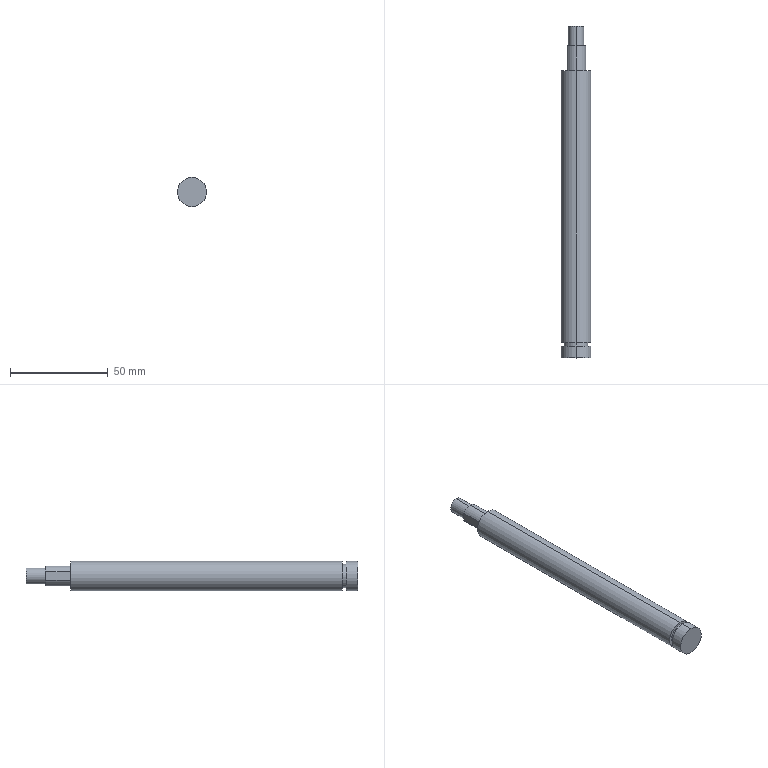Part | SolidWorks | features ICE 1, RevCut 1, Revolution 1 | 1 solid | 18 faces | box 15 x 170 x 15 mm | volume 27374 mm3 | cylinder 11 | plane 7 | commonest cylinder face diameters 15 x4 10 x3 8 x2 12 x2
STEP:
#1=CARTESIAN_POINT('',(0.,6.,7.5));
#2=VERTEX_POINT('',#1);
#3=CARTESIAN_POINT('',(0.,6.,-7.5));
#4=VERTEX_POINT('',#3);
#5=CARTESIAN_POINT('',(0.,6.,0.));
#6=DIRECTION('',(0.,1.,0.));
#7=DIRECTION('',(0.,0.,-1.));
#8=AXIS2_PLACEMENT_3D('',#5,#6,#7);
#9=CIRCLE('',#8,7.5);
#10=EDGE_CURVE('',#2,#4,#9,.T.);
#11=ORIENTED_EDGE('',*,*,#10,.F.);
#12=CARTESIAN_POINT('',(0.,0.,7.5));
#13=VERTEX_POINT('',#12);
#14=CARTESIAN_POINT('',(0.,-11.255,7.5));
#15=DIRECTION('',(0.,-1.,0.));
#16=VECTOR('',#15,1000.);
#17=LINE('',#14,#16);
#18=EDGE_CURVE('',#2,#13,#17,.T.);
#19=ORIENTED_EDGE('',*,*,#18,.T.);
#20=CARTESIAN_POINT('',(0.,0.,-7.5));
#21=VERTEX_POINT('',#20);
#22=CARTESIAN_POINT('',(0.,0.,0.));
#23=DIRECTION('',(0.,-1.,0.));
#24=DIRECTION('',(0.,0.,-1.));
#25=AXIS2_PLACEMENT_3D('',#22,#23,#24);
#26=CIRCLE('',#25,7.5);
#27=EDGE_CURVE('',#21,#13,#26,.T.);
#28=ORIENTED_EDGE('',*,*,#27,.F.);
#29=CARTESIAN_POINT('',(0.,-11.255,-7.5));
#30=DIRECTION('',(0.,-1.,0.));
#31=VECTOR('',#30,1000.);
#32=LINE('',#29,#31);
#33=EDGE_CURVE('',#4,#21,#32,.T.);
#34=ORIENTED_EDGE('',*,*,#33,.F.);
#35=EDGE_LOOP('',(#11,#19,#28,#34));
#36=FACE_OUTER_BOUND('',#35,.T.);
#37=CARTESIAN_POINT('',(0.,-11.255,0.));
#38=DIRECTION('',(0.,-1.,0.));
#39=DIRECTION('',(0.,0.,-1.));
#40=AXIS2_PLACEMENT_3D('',#37,#38,#39);
#41=CYLINDRICAL_SURFACE('',#40,7.5);
#42=ADVANCED_FACE('',(#36),#41,.T.);
#43=CARTESIAN_POINT('',(0.,8.,-6.));
#44=VERTEX_POINT('',#43);
#45=CARTESIAN_POINT('',(0.,8.,6.));
#46=VERTEX_POINT('',#45);
#47=CARTESIAN_POINT('',(0.,8.,0.));
#48=DIRECTION('',(0.,-1.,0.));
#49=DIRECTION('',(0.,0.,-1.));
#50=AXIS2_PLACEMENT_3D('',#47,#48,#49);
#51=CIRCLE('',#50,6.);
#52=EDGE_CURVE('',#44,#46,#51,.T.);
#53=ORIENTED_EDGE('',*,*,#52,.T.);
#54=CARTESIAN_POINT('',(0.,6.,6.));
#55=VERTEX_POINT('',#54);
#56=CARTESIAN_POINT('',(0.,0.,6.));
#57=DIRECTION('',(0.,-1.,0.));
#58=VECTOR('',#57,1000.);
#59=LINE('',#56,#58);
#60=EDGE_CURVE('',#46,#55,#59,.T.);
#61=ORIENTED_EDGE('',*,*,#60,.T.);
#62=CARTESIAN_POINT('',(0.,6.,-6.));
#63=VERTEX_POINT('',#62);
#64=CARTESIAN_POINT('',(0.,6.,0.));
#65=DIRECTION('',(0.,-1.,0.));
#66=DIRECTION('',(0.,0.,-1.));
#67=AXIS2_PLACEMENT_3D('',#64,#65,#66);
#68=CIRCLE('',#67,6.);
#69=EDGE_CURVE('',#63,#55,#68,.T.);
#70=ORIENTED_EDGE('',*,*,#69,.F.);
#71=CARTESIAN_POINT('',(0.,0.,-6.));
#72=DIRECTION('',(0.,-1.,0.));
#73=VECTOR('',#72,1000.);
#74=LINE('',#71,#73);
#75=EDGE_CURVE('',#44,#63,#74,.T.);
#76=ORIENTED_EDGE('',*,*,#75,.F.);
#77=EDGE_LOOP('',(#53,#61,#70,#76));
#78=FACE_OUTER_BOUND('',#77,.T.);
#79=CARTESIAN_POINT('',(0.,0.,0.));
#80=DIRECTION('',(0.,-1.,0.));
#81=DIRECTION('',(0.,0.,-1.));
#82=AXIS2_PLACEMENT_3D('',#79,#80,#81);
#83=CYLINDRICAL_SURFACE('',#82,6.);
#84=ADVANCED_FACE('',(#78),#83,.T.);
#85=CARTESIAN_POINT('',(0.,170.,-4.));
#86=VERTEX_POINT('',#85);
#87=CARTESIAN_POINT('',(0.,170.,4.));
#88=VERTEX_POINT('',#87);
#89=CARTESIAN_POINT('',(0.,170.,0.));
#90=DIRECTION('',(0.,-1.,0.));
#91=DIRECTION('',(0.,0.,-1.));
#92=AXIS2_PLACEMENT_3D('',#89,#90,#91);
#93=CIRCLE('',#92,4.);
#94=EDGE_CURVE('',#86,#88,#93,.T.);
#95=ORIENTED_EDGE('',*,*,#94,.T.);
#96=CARTESIAN_POINT('',(0.,160.,4.));
#97=VERTEX_POINT('',#96);
#98=CARTESIAN_POINT('',(0.,-11.255,4.));
#99=DIRECTION('',(0.,-1.,0.));
#100=VECTOR('',#99,1000.);
#101=LINE('',#98,#100);
#102=EDGE_CURVE('',#88,#97,#101,.T.);
#103=ORIENTED_EDGE('',*,*,#102,.T.);
#104=CARTESIAN_POINT('',(0.,160.,-4.));
#105=VERTEX_POINT('',#104);
#106=CARTESIAN_POINT('',(0.,160.,0.));
#107=DIRECTION('',(0.,-1.,0.));
#108=DIRECTION('',(0.,0.,-1.));
#109=AXIS2_PLACEMENT_3D('',#106,#107,#108);
#110=CIRCLE('',#109,4.);
#111=EDGE_CURVE('',#105,#97,#110,.T.);
#112=ORIENTED_EDGE('',*,*,#111,.F.);
#113=CARTESIAN_POINT('',(0.,-11.255,-4.));
#114=DIRECTION('',(0.,-1.,0.));
#115=VECTOR('',#114,1000.);
#116=LINE('',#113,#115);
#117=EDGE_CURVE('',#86,#105,#116,.T.);
#118=ORIENTED_EDGE('',*,*,#117,.F.);
#119=EDGE_LOOP('',(#95,#103,#112,#118));
#120=FACE_OUTER_BOUND('',#119,.T.);
#121=CARTESIAN_POINT('',(0.,-11.255,0.));
#122=DIRECTION('',(0.,-1.,0.));
#123=DIRECTION('',(0.,0.,-1.));
#124=AXIS2_PLACEMENT_3D('',#121,#122,#123);
#125=CYLINDRICAL_SURFACE('',#124,4.);
#126=ADVANCED_FACE('',(#120),#125,.T.);
#127=CARTESIAN_POINT('',(0.,160.,-5.));
#128=VERTEX_POINT('',#127);
#129=CARTESIAN_POINT('',(0.,160.,5.));
#130=VERTEX_POINT('',#129);
#131=CARTESIAN_POINT('',(0.,160.,0.));
#132=DIRECTION('',(0.,-1.,0.));
#133=DIRECTION('',(0.,0.,-1.));
#134=AXIS2_PLACEMENT_3D('',#131,#132,#133);
#135=CIRCLE('',#134,5.);
#136=EDGE_CURVE('',#128,#130,#135,.T.);
#137=ORIENTED_EDGE('',*,*,#136,.T.);
#138=CARTESIAN_POINT('',(0.,147.2,5.));
#139=VERTEX_POINT('',#138);
#140=CARTESIAN_POINT('',(0.,-11.255,5.));
#141=DIRECTION('',(0.,-1.,0.));
#142=VECTOR('',#141,1000.);
#143=LINE('',#140,#142);
#144=EDGE_CURVE('',#130,#139,#143,.T.);
#145=ORIENTED_EDGE('',*,*,#144,.T.);
#146=CARTESIAN_POINT('',(0.,147.2,-5.));
#147=VERTEX_POINT('',#146);
#148=CARTESIAN_POINT('',(0.,147.2,0.));
#149=DIRECTION('',(0.,-1.,0.));
#150=DIRECTION('',(0.,0.,-1.));
#151=AXIS2_PLACEMENT_3D('',#148,#149,#150);
#152=CIRCLE('',#151,5.);
#153=EDGE_CURVE('',#147,#139,#152,.T.);
#154=ORIENTED_EDGE('',*,*,#153,.F.);
#155=CARTESIAN_POINT('',(0.,-11.255,-5.));
#156=DIRECTION('',(0.,-1.,0.));
#157=VECTOR('',#156,1000.);
#158=LINE('',#155,#157);
#159=EDGE_CURVE('',#128,#147,#158,.T.);
#160=ORIENTED_EDGE('',*,*,#159,.F.);
#161=EDGE_LOOP('',(#137,#145,#154,#160));
#162=FACE_OUTER_BOUND('',#161,.T.);
#163=CARTESIAN_POINT('',(0.,-11.255,0.));
#164=DIRECTION('',(0.,-1.,0.));
#165=DIRECTION('',(0.,0.,-1.));
#166=AXIS2_PLACEMENT_3D('',#163,#164,#165);
#167=CYLINDRICAL_SURFACE('',#166,5.);
#168=ADVANCED_FACE('',(#162),#167,.T.);
#169=CARTESIAN_POINT('',(-4.5,160.,-2.179));
#170=VERTEX_POINT('',#169);
#171=CARTESIAN_POINT('',(0.,160.,0.));
#172=DIRECTION('',(0.,-1.,0.));
#173=DIRECTION('',(0.,0.,-1.));
#174=AXIS2_PLACEMENT_3D('',#171,#172,#173);
#175=CIRCLE('',#174,5.);
#176=EDGE_CURVE('',#170,#128,#175,.T.);
#177=ORIENTED_EDGE('',*,*,#176,.T.);
#178=ORIENTED_EDGE('',*,*,#159,.T.);
#179=CARTESIAN_POINT('',(-4.5,147.2,-2.179));
#180=VERTEX_POINT('',#179);
#181=CARTESIAN_POINT('',(0.,147.2,0.));
#182=DIRECTION('',(0.,-1.,0.));
#183=DIRECTION('',(0.,0.,-1.));
#184=AXIS2_PLACEMENT_3D('',#181,#182,#183);
#185=CIRCLE('',#184,5.);
#186=EDGE_CURVE('',#180,#147,#185,.T.);
#187=ORIENTED_EDGE('',*,*,#186,.F.);
#188=CARTESIAN_POINT('',(-4.5,-11.255,-2.179));
#189=DIRECTION('',(0.,-1.,0.));
#190=VECTOR('',#189,1000.);
#191=LINE('',#188,#190);
#192=EDGE_CURVE('',#170,#180,#191,.T.);
#193=ORIENTED_EDGE('',*,*,#192,.F.);
#194=EDGE_LOOP('',(#177,#178,#187,#193));
#195=FACE_OUTER_BOUND('',#194,.T.);
#196=CARTESIAN_POINT('',(0.,-11.255,0.));
#197=DIRECTION('',(0.,-1.,0.));
#198=DIRECTION('',(0.,0.,-1.));
#199=AXIS2_PLACEMENT_3D('',#196,#197,#198);
#200=CYLINDRICAL_SURFACE('',#199,5.);
#201=ADVANCED_FACE('',(#195),#200,.T.);
#202=CARTESIAN_POINT('',(0.,147.2,-7.5));
#203=VERTEX_POINT('',#202);
#204=CARTESIAN_POINT('',(0.,147.2,7.5));
#205=VERTEX_POINT('',#204);
#206=CARTESIAN_POINT('',(0.,147.2,0.));
#207=DIRECTION('',(0.,-1.,0.));
#208=DIRECTION('',(0.,0.,-1.));
#209=AXIS2_PLACEMENT_3D('',#206,#207,#208);
#210=CIRCLE('',#209,7.5);
#211=EDGE_CURVE('',#203,#205,#210,.T.);
#212=ORIENTED_EDGE('',*,*,#211,.T.);
#213=CARTESIAN_POINT('',(0.,8.,7.5));
#214=VERTEX_POINT('',#213);
#215=CARTESIAN_POINT('',(0.,-11.255,7.5));
#216=DIRECTION('',(0.,-1.,0.));
#217=VECTOR('',#216,1000.);
#218=LINE('',#215,#217);
#219=EDGE_CURVE('',#205,#214,#218,.T.);
#220=ORIENTED_EDGE('',*,*,#219,.T.);
#221=CARTESIAN_POINT('',(0.,8.,-7.5));
#222=VERTEX_POINT('',#221);
#223=CARTESIAN_POINT('',(0.,8.,0.));
#224=DIRECTION('',(0.,-1.,0.));
#225=DIRECTION('',(0.,0.,1.));
#226=AXIS2_PLACEMENT_3D('',#223,#224,#225);
#227=CIRCLE('',#226,7.5);
#228=EDGE_CURVE('',#222,#214,#227,.T.);
#229=ORIENTED_EDGE('',*,*,#228,.F.);
#230=CARTESIAN_POINT('',(0.,-11.255,-7.5));
#231=DIRECTION('',(0.,-1.,0.));
#232=VECTOR('',#231,1000.);
#233=LINE('',#230,#232);
#234=EDGE_CURVE('',#203,#222,#233,.T.);
#235=ORIENTED_EDGE('',*,*,#234,.F.);
#236=EDGE_LOOP('',(#212,#220,#229,#235));
#237=FACE_OUTER_BOUND('',#236,.T.);
#238=CARTESIAN_POINT('',(0.,-11.255,0.));
#239=DIRECTION('',(0.,-1.,0.));
#240=DIRECTION('',(0.,0.,-1.));
#241=AXIS2_PLACEMENT_3D('',#238,#239,#240);
#242=CYLINDRICAL_SURFACE('',#241,7.5);
#243=ADVANCED_FACE('',(#237),#242,.T.);
#244=ORIENTED_EDGE('',*,*,#219,.F.);
#245=CARTESIAN_POINT('',(0.,147.2,0.));
#246=DIRECTION('',(0.,-1.,0.));
#247=DIRECTION('',(0.,0.,-1.));
#248=AXIS2_PLACEMENT_3D('',#245,#246,#247);
#249=CIRCLE('',#248,7.5);
#250=EDGE_CURVE('',#205,#203,#249,.T.);
#251=ORIENTED_EDGE('',*,*,#250,.T.);
#252=ORIENTED_EDGE('',*,*,#234,.T.);
#253=CARTESIAN_POINT('',(0.,8.,0.));
#254=DIRECTION('',(0.,-1.,0.));
#255=DIRECTION('',(0.,0.,1.));
#256=AXIS2_PLACEMENT_3D('',#253,#254,#255);
#257=CIRCLE('',#256,7.5);
#258=EDGE_CURVE('',#214,#222,#257,.T.);
#259=ORIENTED_EDGE('',*,*,#258,.F.);
#260=EDGE_LOOP('',(#244,#251,#252,#259));
#261=FACE_OUTER_BOUND('',#260,.T.);
#262=CARTESIAN_POINT('',(0.,-11.255,0.));
#263=DIRECTION('',(0.,-1.,0.));
#264=DIRECTION('',(0.,0.,-1.));
#265=AXIS2_PLACEMENT_3D('',#262,#263,#264);
#266=CYLINDRICAL_SURFACE('',#265,7.5);
#267=ADVANCED_FACE('',(#261),#266,.T.);
#268=ORIENTED_EDGE('',*,*,#186,.T.);
#269=ORIENTED_EDGE('',*,*,#153,.T.);
#270=CARTESIAN_POINT('',(-4.5,147.2,2.179));
#271=VERTEX_POINT('',#270);
#272=CARTESIAN_POINT('',(0.,147.2,0.));
#273=DIRECTION('',(0.,-1.,0.));
#274=DIRECTION('',(0.,0.,-1.));
#275=AXIS2_PLACEMENT_3D('',#272,#273,#274);
#276=CIRCLE('',#275,5.);
#277=EDGE_CURVE('',#139,#271,#276,.T.);
#278=ORIENTED_EDGE('',*,*,#277,.T.);
#279=CARTESIAN_POINT('',(-4.5,147.2,8.535));
#280=DIRECTION('',(0.,0.,1.));
#281=VECTOR('',#280,1000.);
#282=LINE('',#279,#281);
#283=EDGE_CURVE('',#180,#271,#282,.T.);
#284=ORIENTED_EDGE('',*,*,#283,.F.);
#285=EDGE_LOOP('',(#268,#269,#278,#284));
#286=FACE_BOUND('',#285,.T.);
#287=ORIENTED_EDGE('',*,*,#211,.F.);
#288=ORIENTED_EDGE('',*,*,#250,.F.);
#289=EDGE_LOOP('',(#287,#288));
#290=FACE_OUTER_BOUND('',#289,.T.);
#291=CARTESIAN_POINT('',(7.5,147.2,0.));
#292=DIRECTION('',(0.,1.,0.));
#293=DIRECTION('',(0.,0.,1.));
#294=AXIS2_PLACEMENT_3D('',#291,#292,#293);
#295=PLANE('',#294);
#296=ADVANCED_FACE('',(#286,#290),#295,.T.);
#297=ORIENTED_EDGE('',*,*,#144,.F.);
#298=CARTESIAN_POINT('',(-4.5,160.,2.179));
#299=VERTEX_POINT('',#298);
#300=CARTESIAN_POINT('',(0.,160.,0.));
#301=DIRECTION('',(0.,-1.,0.));
#302=DIRECTION('',(0.,0.,-1.));
#303=AXIS2_PLACEMENT_3D('',#300,#301,#302);
#304=CIRCLE('',#303,5.);
#305=EDGE_CURVE('',#130,#299,#304,.T.);
#306=ORIENTED_EDGE('',*,*,#305,.T.);
#307=CARTESIAN_POINT('',(-4.5,-11.255,2.179));
#308=DIRECTION('',(0.,1.,0.));
#309=VECTOR('',#308,1000.);
#310=LINE('',#307,#309);
#311=EDGE_CURVE('',#271,#299,#310,.T.);
#312=ORIENTED_EDGE('',*,*,#311,.F.);
#313=ORIENTED_EDGE('',*,*,#277,.F.);
#314=EDGE_LOOP('',(#297,#306,#312,#313));
#315=FACE_OUTER_BOUND('',#314,.T.);
#316=CARTESIAN_POINT('',(0.,-11.255,0.));
#317=DIRECTION('',(0.,-1.,0.));
#318=DIRECTION('',(0.,0.,-1.));
#319=AXIS2_PLACEMENT_3D('',#316,#317,#318);
#320=CYLINDRICAL_SURFACE('',#319,5.);
#321=ADVANCED_FACE('',(#315),#320,.T.);
#322=CARTESIAN_POINT('',(-4.5,160.,0.));
#323=DIRECTION('',(0.,0.,-1.));
#324=VECTOR('',#323,1000.);
#325=LINE('',#322,#324);
#326=EDGE_CURVE('',#299,#170,#325,.T.);
#327=ORIENTED_EDGE('',*,*,#326,.F.);
#328=ORIENTED_EDGE('',*,*,#305,.F.);
#329=ORIENTED_EDGE('',*,*,#136,.F.);
#330=ORIENTED_EDGE('',*,*,#176,.F.);
#331=EDGE_LOOP('',(#327,#328,#329,#330));
#332=FACE_OUTER_BOUND('',#331,.T.);
#333=ORIENTED_EDGE('',*,*,#111,.T.);
#334=CARTESIAN_POINT('',(0.,160.,0.));
#335=DIRECTION('',(0.,-1.,0.));
#336=DIRECTION('',(0.,0.,-1.));
#337=AXIS2_PLACEMENT_3D('',#334,#335,#336);
#338=CIRCLE('',#337,4.);
#339=EDGE_CURVE('',#97,#105,#338,.T.);
#340=ORIENTED_EDGE('',*,*,#339,.T.);
#341=EDGE_LOOP('',(#333,#340));
#342=FACE_BOUND('',#341,.T.);
#343=CARTESIAN_POINT('',(5.,160.,0.));
#344=DIRECTION('',(0.,1.,0.));
#345=DIRECTION('',(0.,0.,1.));
#346=AXIS2_PLACEMENT_3D('',#343,#344,#345);
#347=PLANE('',#346);
#348=ADVANCED_FACE('',(#332,#342),#347,.T.);
#349=ORIENTED_EDGE('',*,*,#102,.F.);
#350=CARTESIAN_POINT('',(0.,170.,0.));
#351=DIRECTION('',(0.,-1.,0.));
#352=DIRECTION('',(0.,0.,-1.));
#353=AXIS2_PLACEMENT_3D('',#350,#351,#352);
#354=CIRCLE('',#353,4.);
#355=EDGE_CURVE('',#88,#86,#354,.T.);
#356=ORIENTED_EDGE('',*,*,#355,.T.);
#357=ORIENTED_EDGE('',*,*,#117,.T.);
#358=ORIENTED_EDGE('',*,*,#339,.F.);
#359=EDGE_LOOP('',(#349,#356,#357,#358));
#360=FACE_OUTER_BOUND('',#359,.T.);
#361=CARTESIAN_POINT('',(0.,-11.255,0.));
#362=DIRECTION('',(0.,-1.,0.));
#363=DIRECTION('',(0.,0.,-1.));
#364=AXIS2_PLACEMENT_3D('',#361,#362,#363);
#365=CYLINDRICAL_SURFACE('',#364,4.);
#366=ADVANCED_FACE('',(#360),#365,.T.);
#367=ORIENTED_EDGE('',*,*,#94,.F.);
#368=ORIENTED_EDGE('',*,*,#355,.F.);
#369=EDGE_LOOP('',(#367,#368));
#370=FACE_OUTER_BOUND('',#369,.T.);
#371=CARTESIAN_POINT('',(4.,170.,0.));
#372=DIRECTION('',(0.,1.,0.));
#373=DIRECTION('',(0.,0.,1.));
#374=AXIS2_PLACEMENT_3D('',#371,#372,#373);
#375=PLANE('',#374);
#376=ADVANCED_FACE('',(#370),#375,.T.);
#377=ORIENTED_EDGE('',*,*,#311,.T.);
#378=ORIENTED_EDGE('',*,*,#326,.T.);
#379=ORIENTED_EDGE('',*,*,#192,.T.);
#380=ORIENTED_EDGE('',*,*,#283,.T.);
#381=EDGE_LOOP('',(#377,#378,#379,#380));
#382=FACE_OUTER_BOUND('',#381,.T.);
#383=CARTESIAN_POINT('',(-4.5,131.486,8.535));
#384=DIRECTION('',(1.,0.,0.));
#385=DIRECTION('',(0.,0.,-1.));
#386=AXIS2_PLACEMENT_3D('',#383,#384,#385);
#387=PLANE('',#386);
#388=ADVANCED_FACE('',(#382),#387,.F.);
#389=ORIENTED_EDGE('',*,*,#60,.F.);
#390=CARTESIAN_POINT('',(0.,8.,0.));
#391=DIRECTION('',(0.,-1.,0.));
#392=DIRECTION('',(0.,0.,-1.));
#393=AXIS2_PLACEMENT_3D('',#390,#391,#392);
#394=CIRCLE('',#393,6.);
#395=EDGE_CURVE('',#46,#44,#394,.T.);
#396=ORIENTED_EDGE('',*,*,#395,.T.);
#397=ORIENTED_EDGE('',*,*,#75,.T.);
#398=CARTESIAN_POINT('',(0.,6.,0.));
#399=DIRECTION('',(0.,-1.,0.));
#400=DIRECTION('',(0.,0.,-1.));
#401=AXIS2_PLACEMENT_3D('',#398,#399,#400);
#402=CIRCLE('',#401,6.);
#403=EDGE_CURVE('',#55,#63,#402,.T.);
#404=ORIENTED_EDGE('',*,*,#403,.F.);
#405=EDGE_LOOP('',(#389,#396,#397,#404));
#406=FACE_OUTER_BOUND('',#405,.T.);
#407=CARTESIAN_POINT('',(0.,0.,0.));
#408=DIRECTION('',(0.,-1.,0.));
#409=DIRECTION('',(0.,0.,-1.));
#410=AXIS2_PLACEMENT_3D('',#407,#408,#409);
#411=CYLINDRICAL_SURFACE('',#410,6.);
#412=ADVANCED_FACE('',(#406),#411,.T.);
#413=ORIENTED_EDGE('',*,*,#228,.T.);
#414=ORIENTED_EDGE('',*,*,#258,.T.);
#415=EDGE_LOOP('',(#413,#414));
#416=FACE_OUTER_BOUND('',#415,.T.);
#417=ORIENTED_EDGE('',*,*,#52,.F.);
#418=ORIENTED_EDGE('',*,*,#395,.F.);
#419=EDGE_LOOP('',(#417,#418));
#420=FACE_BOUND('',#419,.T.);
#421=CARTESIAN_POINT('',(6.,8.,0.));
#422=DIRECTION('',(0.,1.,0.));
#423=DIRECTION('',(0.,0.,1.));
#424=AXIS2_PLACEMENT_3D('',#421,#422,#423);
#425=PLANE('',#424);
#426=ADVANCED_FACE('',(#416,#420),#425,.F.);
#427=CARTESIAN_POINT('',(0.,6.,0.));
#428=DIRECTION('',(0.,1.,0.));
#429=DIRECTION('',(0.,0.,-1.));
#430=AXIS2_PLACEMENT_3D('',#427,#428,#429);
#431=CIRCLE('',#430,7.5);
#432=EDGE_CURVE('',#4,#2,#431,.T.);
#433=ORIENTED_EDGE('',*,*,#432,.T.);
#434=ORIENTED_EDGE('',*,*,#10,.T.);
#435=EDGE_LOOP('',(#433,#434));
#436=FACE_OUTER_BOUND('',#435,.T.);
#437=ORIENTED_EDGE('',*,*,#69,.T.);
#438=ORIENTED_EDGE('',*,*,#403,.T.);
#439=EDGE_LOOP('',(#437,#438));
#440=FACE_BOUND('',#439,.T.);
#441=CARTESIAN_POINT('',(6.,6.,0.));
#442=DIRECTION('',(0.,-1.,0.));
#443=DIRECTION('',(0.,0.,-1.));
#444=AXIS2_PLACEMENT_3D('',#441,#442,#443);
#445=PLANE('',#444);
#446=ADVANCED_FACE('',(#436,#440),#445,.F.);
#447=ORIENTED_EDGE('',*,*,#27,.T.);
#448=CARTESIAN_POINT('',(0.,0.,0.));
#449=DIRECTION('',(0.,-1.,0.));
#450=DIRECTION('',(0.,0.,-1.));
#451=AXIS2_PLACEMENT_3D('',#448,#449,#450);
#452=CIRCLE('',#451,7.5);
#453=EDGE_CURVE('',#13,#21,#452,.T.);
#454=ORIENTED_EDGE('',*,*,#453,.T.);
#455=EDGE_LOOP('',(#447,#454));
#456=FACE_OUTER_BOUND('',#455,.T.);
#457=CARTESIAN_POINT('',(0.,0.,0.));
#458=DIRECTION('',(0.,-1.,0.));
#459=DIRECTION('',(0.,0.,-1.));
#460=AXIS2_PLACEMENT_3D('',#457,#458,#459);
#461=PLANE('',#460);
#462=ADVANCED_FACE('',(#456),#461,.T.);
#463=ORIENTED_EDGE('',*,*,#18,.F.);
#464=ORIENTED_EDGE('',*,*,#432,.F.);
#465=ORIENTED_EDGE('',*,*,#33,.T.);
#466=ORIENTED_EDGE('',*,*,#453,.F.);
#467=EDGE_LOOP('',(#463,#464,#465,#466));
#468=FACE_OUTER_BOUND('',#467,.T.);
#469=CARTESIAN_POINT('',(0.,-11.255,0.));
#470=DIRECTION('',(0.,-1.,0.));
#471=DIRECTION('',(0.,0.,-1.));
#472=AXIS2_PLACEMENT_3D('',#469,#470,#471);
#473=CYLINDRICAL_SURFACE('',#472,7.5);
#474=ADVANCED_FACE('',(#468),#473,.T.);
#475=CLOSED_SHELL('',(#42,#84,#126,#168,#201,#243,#267,#296,#321,#348,#366,#376,#388,#412,#426,#446,#462,#474));
#476=MANIFOLD_SOLID_BREP('',#475);
#477=CARTESIAN_POINT('',(0.,0.,0.));
#478=DIRECTION('',(0.,0.,1.));
#479=DIRECTION('',(1.,0.,0.));
#480=AXIS2_PLACEMENT_3D('',#477,#478,#479);
#481=(LENGTH_UNIT()NAMED_UNIT(*)SI_UNIT(.MILLI.,.METRE.));
#482=UNCERTAINTY_MEASURE_WITH_UNIT(LENGTH_MEASURE(0.00001),#481,'','');
#483=(NAMED_UNIT(*)PLANE_ANGLE_UNIT()SI_UNIT($,.RADIAN.));
#484=(NAMED_UNIT(*)SI_UNIT($,.STERADIAN.)SOLID_ANGLE_UNIT());
#485=(GEOMETRIC_REPRESENTATION_CONTEXT(3)GLOBAL_UNCERTAINTY_ASSIGNED_CONTEXT((#482))GLOBAL_UNIT_ASSIGNED_CONTEXT((#481,#483,#484))REPRESENTATION_CONTEXT('',''));
#486=ADVANCED_BREP_SHAPE_REPRESENTATION('',(#476,#480),#485);